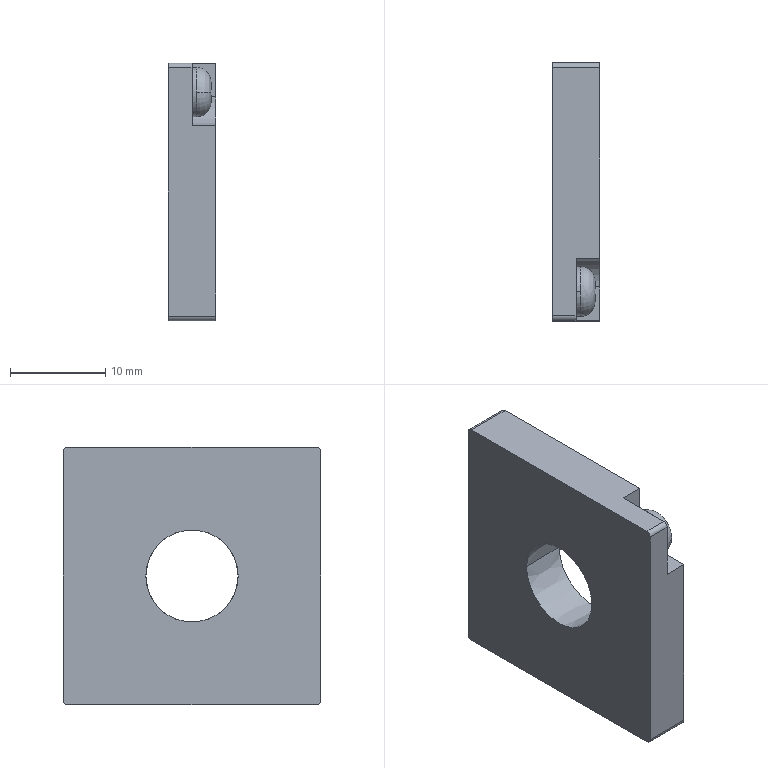Part | STEP file | 1 solid | 62 faces | box 5 x 27.1 x 27.1 mm | volume 3152 mm3 | plane 46 | cylinder 10 | other 4 | cone 2 | commonest cylinder face diameters 1 x4 5.2 x4 6 x2